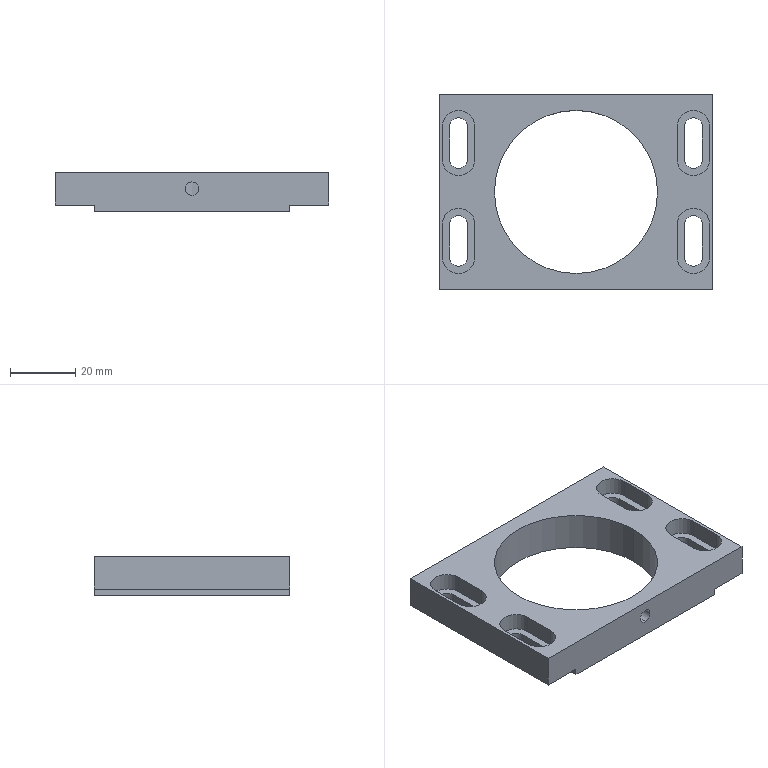Part | SolidWorks | features HoleWzd 2, ICE 2, Extrusion 1 | 1 solid | 50 faces | box 84 x 60 x 12 mm | volume 28663 mm3 | plane 30 | cylinder 20 | commonest cylinder face diameters 5.5 x8 10 x8 4.2 x2 50 x2